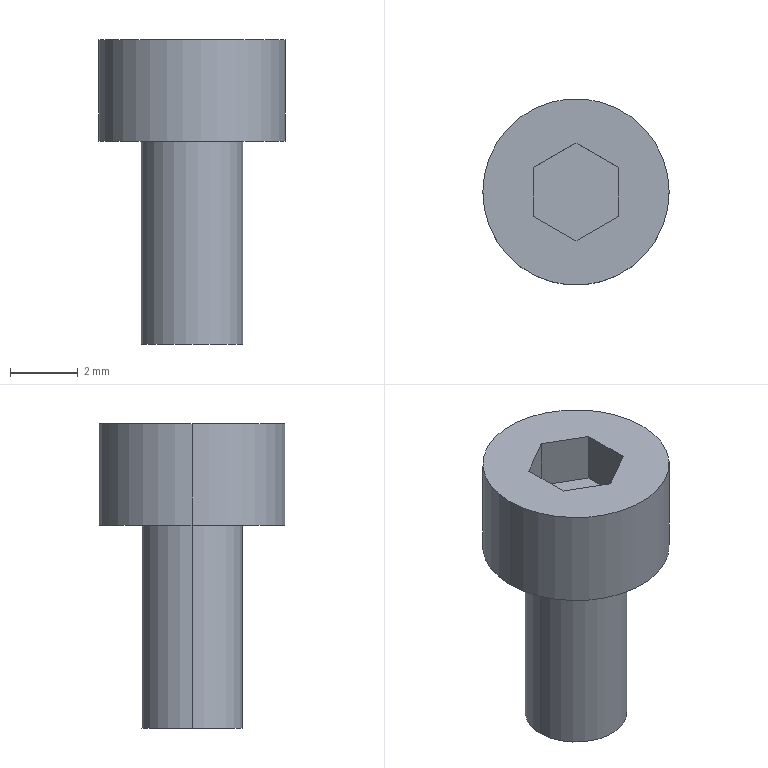Part | STEP file | QCTHA0834-14_03^qctha0834-14_FBDS-CS | 1 solid | 14 faces | box 5.5 x 5.5 x 9 mm | volume 105.567 mm3 | plane 10 | cylinder 4 | commonest cylinder face diameters 3 x2 5.5 x2
STEP:
#1=CARTESIAN_POINT('',(1.5,0.,-6.));
#2=VERTEX_POINT('',#1);
#3=CARTESIAN_POINT('',(-1.5,0.,-6.));
#4=VERTEX_POINT('',#3);
#5=CARTESIAN_POINT('',(0.,0.,-6.));
#6=DIRECTION('',(0.,0.,1.));
#7=DIRECTION('',(1.,0.,0.));
#8=AXIS2_PLACEMENT_3D('',#5,#6,#7);
#9=CIRCLE('',#8,1.5);
#10=EDGE_CURVE('',#2,#4,#9,.T.);
#11=ORIENTED_EDGE('',*,*,#10,.T.);
#12=CARTESIAN_POINT('',(-1.5,0.,0.));
#13=VERTEX_POINT('',#12);
#14=CARTESIAN_POINT('',(-1.5,0.,14.));
#15=DIRECTION('',(0.,0.,1.));
#16=VECTOR('',#15,1000.);
#17=LINE('',#14,#16);
#18=EDGE_CURVE('',#4,#13,#17,.T.);
#19=ORIENTED_EDGE('',*,*,#18,.T.);
#20=CARTESIAN_POINT('',(1.5,0.,0.));
#21=VERTEX_POINT('',#20);
#22=CARTESIAN_POINT('',(0.,0.,0.));
#23=DIRECTION('',(0.,0.,1.));
#24=DIRECTION('',(1.,0.,0.));
#25=AXIS2_PLACEMENT_3D('',#22,#23,#24);
#26=CIRCLE('',#25,1.5);
#27=EDGE_CURVE('',#21,#13,#26,.T.);
#28=ORIENTED_EDGE('',*,*,#27,.F.);
#29=CARTESIAN_POINT('',(1.5,0.,14.));
#30=DIRECTION('',(0.,0.,1.));
#31=VECTOR('',#30,1000.);
#32=LINE('',#29,#31);
#33=EDGE_CURVE('',#2,#21,#32,.T.);
#34=ORIENTED_EDGE('',*,*,#33,.F.);
#35=EDGE_LOOP('',(#11,#19,#28,#34));
#36=FACE_OUTER_BOUND('',#35,.T.);
#37=CARTESIAN_POINT('',(0.,0.,14.));
#38=DIRECTION('',(0.,0.,1.));
#39=DIRECTION('',(1.,0.,0.));
#40=AXIS2_PLACEMENT_3D('',#37,#38,#39);
#41=CYLINDRICAL_SURFACE('',#40,1.5);
#42=ADVANCED_FACE('',(#36),#41,.T.);
#43=CARTESIAN_POINT('',(2.75,0.,0.));
#44=VERTEX_POINT('',#43);
#45=CARTESIAN_POINT('',(-2.75,0.,0.));
#46=VERTEX_POINT('',#45);
#47=CARTESIAN_POINT('',(0.,0.,0.));
#48=DIRECTION('',(0.,0.,1.));
#49=DIRECTION('',(1.,0.,0.));
#50=AXIS2_PLACEMENT_3D('',#47,#48,#49);
#51=CIRCLE('',#50,2.75);
#52=EDGE_CURVE('',#44,#46,#51,.T.);
#53=ORIENTED_EDGE('',*,*,#52,.T.);
#54=CARTESIAN_POINT('',(-2.75,0.,3.));
#55=VERTEX_POINT('',#54);
#56=CARTESIAN_POINT('',(-2.75,0.,14.));
#57=DIRECTION('',(0.,0.,1.));
#58=VECTOR('',#57,1000.);
#59=LINE('',#56,#58);
#60=EDGE_CURVE('',#46,#55,#59,.T.);
#61=ORIENTED_EDGE('',*,*,#60,.T.);
#62=CARTESIAN_POINT('',(2.75,0.,3.));
#63=VERTEX_POINT('',#62);
#64=CARTESIAN_POINT('',(0.,0.,3.));
#65=DIRECTION('',(0.,0.,1.));
#66=DIRECTION('',(1.,0.,0.));
#67=AXIS2_PLACEMENT_3D('',#64,#65,#66);
#68=CIRCLE('',#67,2.75);
#69=EDGE_CURVE('',#63,#55,#68,.T.);
#70=ORIENTED_EDGE('',*,*,#69,.F.);
#71=CARTESIAN_POINT('',(2.75,0.,14.));
#72=DIRECTION('',(0.,0.,1.));
#73=VECTOR('',#72,1000.);
#74=LINE('',#71,#73);
#75=EDGE_CURVE('',#44,#63,#74,.T.);
#76=ORIENTED_EDGE('',*,*,#75,.F.);
#77=EDGE_LOOP('',(#53,#61,#70,#76));
#78=FACE_OUTER_BOUND('',#77,.T.);
#79=CARTESIAN_POINT('',(0.,0.,14.));
#80=DIRECTION('',(0.,0.,1.));
#81=DIRECTION('',(1.,0.,0.));
#82=AXIS2_PLACEMENT_3D('',#79,#80,#81);
#83=CYLINDRICAL_SURFACE('',#82,2.75);
#84=ADVANCED_FACE('',(#78),#83,.T.);
#85=CARTESIAN_POINT('',(1.25,0.7217,1.5));
#86=VERTEX_POINT('',#85);
#87=CARTESIAN_POINT('',(1.25,0.7217,3.));
#88=VERTEX_POINT('',#87);
#89=CARTESIAN_POINT('',(1.25,0.7217,1.5));
#90=DIRECTION('',(0.,0.,1.));
#91=VECTOR('',#90,1000.);
#92=LINE('',#89,#91);
#93=EDGE_CURVE('',#86,#88,#92,.T.);
#94=ORIENTED_EDGE('',*,*,#93,.T.);
#95=CARTESIAN_POINT('',(0.,1.443,3.));
#96=VERTEX_POINT('',#95);
#97=CARTESIAN_POINT('',(0.,1.443,3.));
#98=DIRECTION('',(0.866,-0.5,0.));
#99=VECTOR('',#98,1000.);
#100=LINE('',#97,#99);
#101=EDGE_CURVE('',#96,#88,#100,.T.);
#102=ORIENTED_EDGE('',*,*,#101,.F.);
#103=CARTESIAN_POINT('',(0.,1.443,1.5));
#104=VERTEX_POINT('',#103);
#105=CARTESIAN_POINT('',(0.,1.443,1.5));
#106=DIRECTION('',(0.,0.,1.));
#107=VECTOR('',#106,1000.);
#108=LINE('',#105,#107);
#109=EDGE_CURVE('',#104,#96,#108,.T.);
#110=ORIENTED_EDGE('',*,*,#109,.F.);
#111=CARTESIAN_POINT('',(0.,1.443,1.5));
#112=DIRECTION('',(0.866,-0.5,0.));
#113=VECTOR('',#112,1000.);
#114=LINE('',#111,#113);
#115=EDGE_CURVE('',#104,#86,#114,.T.);
#116=ORIENTED_EDGE('',*,*,#115,.T.);
#117=EDGE_LOOP('',(#94,#102,#110,#116));
#118=FACE_OUTER_BOUND('',#117,.T.);
#119=CARTESIAN_POINT('',(0.,1.443,1.5));
#120=DIRECTION('',(-0.5,-0.866,0.));
#121=DIRECTION('',(-0.866,0.5,0.));
#122=AXIS2_PLACEMENT_3D('',#119,#120,#121);
#123=PLANE('',#122);
#124=ADVANCED_FACE('',(#118),#123,.T.);
#125=CARTESIAN_POINT('',(1.25,-0.7217,1.5));
#126=VERTEX_POINT('',#125);
#127=CARTESIAN_POINT('',(1.25,-0.7217,3.));
#128=VERTEX_POINT('',#127);
#129=CARTESIAN_POINT('',(1.25,-0.7217,1.5));
#130=DIRECTION('',(0.,0.,1.));
#131=VECTOR('',#130,1000.);
#132=LINE('',#129,#131);
#133=EDGE_CURVE('',#126,#128,#132,.T.);
#134=ORIENTED_EDGE('',*,*,#133,.T.);
#135=CARTESIAN_POINT('',(1.25,-0.7217,3.));
#136=DIRECTION('',(0.,1.,0.));
#137=VECTOR('',#136,1000.);
#138=LINE('',#135,#137);
#139=EDGE_CURVE('',#128,#88,#138,.T.);
#140=ORIENTED_EDGE('',*,*,#139,.T.);
#141=ORIENTED_EDGE('',*,*,#93,.F.);
#142=CARTESIAN_POINT('',(1.25,-0.7217,1.5));
#143=DIRECTION('',(0.,1.,0.));
#144=VECTOR('',#143,1000.);
#145=LINE('',#142,#144);
#146=EDGE_CURVE('',#126,#86,#145,.T.);
#147=ORIENTED_EDGE('',*,*,#146,.F.);
#148=EDGE_LOOP('',(#134,#140,#141,#147));
#149=FACE_OUTER_BOUND('',#148,.T.);
#150=CARTESIAN_POINT('',(1.25,-0.7217,1.5));
#151=DIRECTION('',(1.,0.,0.));
#152=DIRECTION('',(0.,0.,1.));
#153=AXIS2_PLACEMENT_3D('',#150,#151,#152);
#154=PLANE('',#153);
#155=ADVANCED_FACE('',(#149),#154,.F.);
#156=CARTESIAN_POINT('',(0.,-1.443,1.5));
#157=VERTEX_POINT('',#156);
#158=CARTESIAN_POINT('',(0.,-1.443,3.));
#159=VERTEX_POINT('',#158);
#160=CARTESIAN_POINT('',(0.,-1.443,1.5));
#161=DIRECTION('',(0.,0.,1.));
#162=VECTOR('',#161,1000.);
#163=LINE('',#160,#162);
#164=EDGE_CURVE('',#157,#159,#163,.T.);
#165=ORIENTED_EDGE('',*,*,#164,.T.);
#166=CARTESIAN_POINT('',(0.,-1.443,3.));
#167=DIRECTION('',(0.866,0.5,0.));
#168=VECTOR('',#167,1000.);
#169=LINE('',#166,#168);
#170=EDGE_CURVE('',#159,#128,#169,.T.);
#171=ORIENTED_EDGE('',*,*,#170,.T.);
#172=ORIENTED_EDGE('',*,*,#133,.F.);
#173=CARTESIAN_POINT('',(0.,-1.443,1.5));
#174=DIRECTION('',(0.866,0.5,0.));
#175=VECTOR('',#174,1000.);
#176=LINE('',#173,#175);
#177=EDGE_CURVE('',#157,#126,#176,.T.);
#178=ORIENTED_EDGE('',*,*,#177,.F.);
#179=EDGE_LOOP('',(#165,#171,#172,#178));
#180=FACE_OUTER_BOUND('',#179,.T.);
#181=CARTESIAN_POINT('',(0.,-1.443,1.5));
#182=DIRECTION('',(0.5,-0.866,0.));
#183=DIRECTION('',(0.,0.,-1.));
#184=AXIS2_PLACEMENT_3D('',#181,#182,#183);
#185=PLANE('',#184);
#186=ADVANCED_FACE('',(#180),#185,.F.);
#187=CARTESIAN_POINT('',(-1.25,-0.7217,1.5));
#188=VERTEX_POINT('',#187);
#189=CARTESIAN_POINT('',(-1.25,-0.7217,3.));
#190=VERTEX_POINT('',#189);
#191=CARTESIAN_POINT('',(-1.25,-0.7217,1.5));
#192=DIRECTION('',(0.,0.,1.));
#193=VECTOR('',#192,1000.);
#194=LINE('',#191,#193);
#195=EDGE_CURVE('',#188,#190,#194,.T.);
#196=ORIENTED_EDGE('',*,*,#195,.T.);
#197=CARTESIAN_POINT('',(0.,-1.443,3.));
#198=DIRECTION('',(-0.866,0.5,0.));
#199=VECTOR('',#198,1000.);
#200=LINE('',#197,#199);
#201=EDGE_CURVE('',#159,#190,#200,.T.);
#202=ORIENTED_EDGE('',*,*,#201,.F.);
#203=ORIENTED_EDGE('',*,*,#164,.F.);
#204=CARTESIAN_POINT('',(0.,-1.443,1.5));
#205=DIRECTION('',(-0.866,0.5,0.));
#206=VECTOR('',#205,1000.);
#207=LINE('',#204,#206);
#208=EDGE_CURVE('',#157,#188,#207,.T.);
#209=ORIENTED_EDGE('',*,*,#208,.T.);
#210=EDGE_LOOP('',(#196,#202,#203,#209));
#211=FACE_OUTER_BOUND('',#210,.T.);
#212=CARTESIAN_POINT('',(0.,-1.443,1.5));
#213=DIRECTION('',(0.5,0.866,0.));
#214=DIRECTION('',(0.,0.,-1.));
#215=AXIS2_PLACEMENT_3D('',#212,#213,#214);
#216=PLANE('',#215);
#217=ADVANCED_FACE('',(#211),#216,.T.);
#218=CARTESIAN_POINT('',(-1.25,0.7217,1.5));
#219=VERTEX_POINT('',#218);
#220=CARTESIAN_POINT('',(-1.25,0.7217,3.));
#221=VERTEX_POINT('',#220);
#222=CARTESIAN_POINT('',(-1.25,0.7217,1.5));
#223=DIRECTION('',(0.,0.,1.));
#224=VECTOR('',#223,1000.);
#225=LINE('',#222,#224);
#226=EDGE_CURVE('',#219,#221,#225,.T.);
#227=ORIENTED_EDGE('',*,*,#226,.T.);
#228=CARTESIAN_POINT('',(-1.25,0.7217,3.));
#229=DIRECTION('',(0.,-1.,0.));
#230=VECTOR('',#229,1000.);
#231=LINE('',#228,#230);
#232=EDGE_CURVE('',#221,#190,#231,.T.);
#233=ORIENTED_EDGE('',*,*,#232,.T.);
#234=ORIENTED_EDGE('',*,*,#195,.F.);
#235=CARTESIAN_POINT('',(-1.25,0.7217,1.5));
#236=DIRECTION('',(0.,-1.,0.));
#237=VECTOR('',#236,1000.);
#238=LINE('',#235,#237);
#239=EDGE_CURVE('',#219,#188,#238,.T.);
#240=ORIENTED_EDGE('',*,*,#239,.F.);
#241=EDGE_LOOP('',(#227,#233,#234,#240));
#242=FACE_OUTER_BOUND('',#241,.T.);
#243=CARTESIAN_POINT('',(-1.25,0.7217,1.5));
#244=DIRECTION('',(-1.,0.,0.));
#245=DIRECTION('',(0.,0.,1.));
#246=AXIS2_PLACEMENT_3D('',#243,#244,#245);
#247=PLANE('',#246);
#248=ADVANCED_FACE('',(#242),#247,.F.);
#249=ORIENTED_EDGE('',*,*,#115,.F.);
#250=CARTESIAN_POINT('',(0.,1.443,1.5));
#251=DIRECTION('',(-0.866,-0.5,0.));
#252=VECTOR('',#251,1000.);
#253=LINE('',#250,#252);
#254=EDGE_CURVE('',#104,#219,#253,.T.);
#255=ORIENTED_EDGE('',*,*,#254,.T.);
#256=ORIENTED_EDGE('',*,*,#239,.T.);
#257=ORIENTED_EDGE('',*,*,#208,.F.);
#258=ORIENTED_EDGE('',*,*,#177,.T.);
#259=ORIENTED_EDGE('',*,*,#146,.T.);
#260=EDGE_LOOP('',(#249,#255,#256,#257,#258,#259));
#261=FACE_OUTER_BOUND('',#260,.T.);
#262=CARTESIAN_POINT('',(1.25,0.7217,1.5));
#263=DIRECTION('',(0.,0.,1.));
#264=DIRECTION('',(1.,0.,0.));
#265=AXIS2_PLACEMENT_3D('',#262,#263,#264);
#266=PLANE('',#265);
#267=ADVANCED_FACE('',(#261),#266,.T.);
#268=ORIENTED_EDGE('',*,*,#254,.F.);
#269=ORIENTED_EDGE('',*,*,#109,.T.);
#270=CARTESIAN_POINT('',(0.,1.443,3.));
#271=DIRECTION('',(-0.866,-0.5,0.));
#272=VECTOR('',#271,1000.);
#273=LINE('',#270,#272);
#274=EDGE_CURVE('',#96,#221,#273,.T.);
#275=ORIENTED_EDGE('',*,*,#274,.T.);
#276=ORIENTED_EDGE('',*,*,#226,.F.);
#277=EDGE_LOOP('',(#268,#269,#275,#276));
#278=FACE_OUTER_BOUND('',#277,.T.);
#279=CARTESIAN_POINT('',(0.,1.443,1.5));
#280=DIRECTION('',(-0.5,0.866,0.));
#281=DIRECTION('',(0.,0.,1.));
#282=AXIS2_PLACEMENT_3D('',#279,#280,#281);
#283=PLANE('',#282);
#284=ADVANCED_FACE('',(#278),#283,.F.);
#285=ORIENTED_EDGE('',*,*,#69,.T.);
#286=CARTESIAN_POINT('',(0.,0.,3.));
#287=DIRECTION('',(0.,0.,1.));
#288=DIRECTION('',(1.,0.,0.));
#289=AXIS2_PLACEMENT_3D('',#286,#287,#288);
#290=CIRCLE('',#289,2.75);
#291=EDGE_CURVE('',#55,#63,#290,.T.);
#292=ORIENTED_EDGE('',*,*,#291,.T.);
#293=EDGE_LOOP('',(#285,#292));
#294=FACE_OUTER_BOUND('',#293,.T.);
#295=ORIENTED_EDGE('',*,*,#274,.F.);
#296=ORIENTED_EDGE('',*,*,#101,.T.);
#297=ORIENTED_EDGE('',*,*,#139,.F.);
#298=ORIENTED_EDGE('',*,*,#170,.F.);
#299=ORIENTED_EDGE('',*,*,#201,.T.);
#300=ORIENTED_EDGE('',*,*,#232,.F.);
#301=EDGE_LOOP('',(#295,#296,#297,#298,#299,#300));
#302=FACE_BOUND('',#301,.T.);
#303=CARTESIAN_POINT('',(0.,0.,3.));
#304=DIRECTION('',(0.,0.,1.));
#305=DIRECTION('',(1.,0.,0.));
#306=AXIS2_PLACEMENT_3D('',#303,#304,#305);
#307=PLANE('',#306);
#308=ADVANCED_FACE('',(#294,#302),#307,.T.);
#309=ORIENTED_EDGE('',*,*,#60,.F.);
#310=CARTESIAN_POINT('',(0.,0.,0.));
#311=DIRECTION('',(0.,0.,1.));
#312=DIRECTION('',(1.,0.,0.));
#313=AXIS2_PLACEMENT_3D('',#310,#311,#312);
#314=CIRCLE('',#313,2.75);
#315=EDGE_CURVE('',#46,#44,#314,.T.);
#316=ORIENTED_EDGE('',*,*,#315,.T.);
#317=ORIENTED_EDGE('',*,*,#75,.T.);
#318=ORIENTED_EDGE('',*,*,#291,.F.);
#319=EDGE_LOOP('',(#309,#316,#317,#318));
#320=FACE_OUTER_BOUND('',#319,.T.);
#321=CARTESIAN_POINT('',(0.,0.,14.));
#322=DIRECTION('',(0.,0.,1.));
#323=DIRECTION('',(1.,0.,0.));
#324=AXIS2_PLACEMENT_3D('',#321,#322,#323);
#325=CYLINDRICAL_SURFACE('',#324,2.75);
#326=ADVANCED_FACE('',(#320),#325,.T.);
#327=ORIENTED_EDGE('',*,*,#52,.F.);
#328=ORIENTED_EDGE('',*,*,#315,.F.);
#329=EDGE_LOOP('',(#327,#328));
#330=FACE_OUTER_BOUND('',#329,.T.);
#331=ORIENTED_EDGE('',*,*,#27,.T.);
#332=CARTESIAN_POINT('',(0.,0.,0.));
#333=DIRECTION('',(0.,0.,1.));
#334=DIRECTION('',(1.,0.,0.));
#335=AXIS2_PLACEMENT_3D('',#332,#333,#334);
#336=CIRCLE('',#335,1.5);
#337=EDGE_CURVE('',#13,#21,#336,.T.);
#338=ORIENTED_EDGE('',*,*,#337,.T.);
#339=EDGE_LOOP('',(#331,#338));
#340=FACE_BOUND('',#339,.T.);
#341=CARTESIAN_POINT('',(2.75,0.,0.));
#342=DIRECTION('',(0.,0.,-1.));
#343=DIRECTION('',(0.,-1.,0.));
#344=AXIS2_PLACEMENT_3D('',#341,#342,#343);
#345=PLANE('',#344);
#346=ADVANCED_FACE('',(#330,#340),#345,.T.);
#347=ORIENTED_EDGE('',*,*,#18,.F.);
#348=CARTESIAN_POINT('',(0.,0.,-6.));
#349=DIRECTION('',(0.,0.,1.));
#350=DIRECTION('',(1.,0.,0.));
#351=AXIS2_PLACEMENT_3D('',#348,#349,#350);
#352=CIRCLE('',#351,1.5);
#353=EDGE_CURVE('',#4,#2,#352,.T.);
#354=ORIENTED_EDGE('',*,*,#353,.T.);
#355=ORIENTED_EDGE('',*,*,#33,.T.);
#356=ORIENTED_EDGE('',*,*,#337,.F.);
#357=EDGE_LOOP('',(#347,#354,#355,#356));
#358=FACE_OUTER_BOUND('',#357,.T.);
#359=CARTESIAN_POINT('',(0.,0.,14.));
#360=DIRECTION('',(0.,0.,1.));
#361=DIRECTION('',(1.,0.,0.));
#362=AXIS2_PLACEMENT_3D('',#359,#360,#361);
#363=CYLINDRICAL_SURFACE('',#362,1.5);
#364=ADVANCED_FACE('',(#358),#363,.T.);
#365=ORIENTED_EDGE('',*,*,#10,.F.);
#366=ORIENTED_EDGE('',*,*,#353,.F.);
#367=EDGE_LOOP('',(#365,#366));
#368=FACE_OUTER_BOUND('',#367,.T.);
#369=CARTESIAN_POINT('',(1.5,0.,-6.));
#370=DIRECTION('',(0.,0.,-1.));
#371=DIRECTION('',(0.,-1.,0.));
#372=AXIS2_PLACEMENT_3D('',#369,#370,#371);
#373=PLANE('',#372);
#374=ADVANCED_FACE('',(#368),#373,.T.);
#375=CLOSED_SHELL('',(#42,#84,#124,#155,#186,#217,#248,#267,#284,#308,#326,#346,#364,#374));
#376=MANIFOLD_SOLID_BREP('',#375);
#377=CARTESIAN_POINT('',(0.,0.,0.));
#378=DIRECTION('',(0.,0.,1.));
#379=DIRECTION('',(1.,0.,0.));
#380=AXIS2_PLACEMENT_3D('',#377,#378,#379);
#381=(LENGTH_UNIT()NAMED_UNIT(*)SI_UNIT(.MILLI.,.METRE.));
#382=UNCERTAINTY_MEASURE_WITH_UNIT(LENGTH_MEASURE(0.00001),#381,'','');
#383=(NAMED_UNIT(*)PLANE_ANGLE_UNIT()SI_UNIT($,.RADIAN.));
#384=(NAMED_UNIT(*)SI_UNIT($,.STERADIAN.)SOLID_ANGLE_UNIT());
#385=(GEOMETRIC_REPRESENTATION_CONTEXT(3)GLOBAL_UNCERTAINTY_ASSIGNED_CONTEXT((#382))GLOBAL_UNIT_ASSIGNED_CONTEXT((#381,#383,#384))REPRESENTATION_CONTEXT('',''));
#386=ADVANCED_BREP_SHAPE_REPRESENTATION('',(#376,#380),#385);